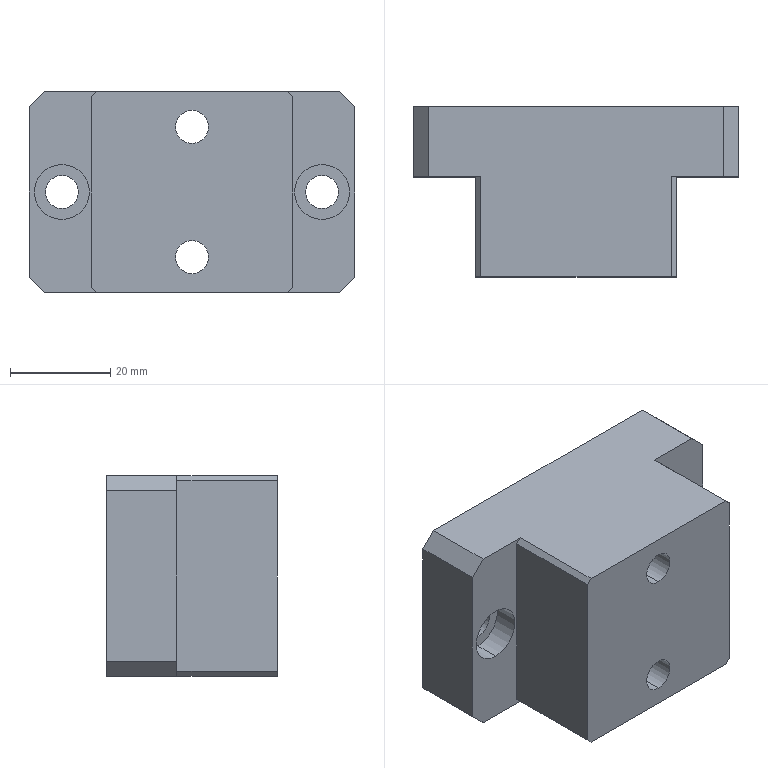Part | SolidWorks | features Chamfer 2, HoleWzd 2, Extrusion 1, ICE 1 | 1 solid | 38 faces | box 65 x 34 x 40 mm | volume 63388 mm3 | plane 22 | cylinder 16 | commonest cylinder face diameters 6.6 x8 11 x8
STEP:
#1=CARTESIAN_POINT('',(26.,8.,5.5));
#2=VERTEX_POINT('',#1);
#3=CARTESIAN_POINT('',(26.,8.,-5.5));
#4=VERTEX_POINT('',#3);
#5=CARTESIAN_POINT('',(26.,8.,0.));
#6=DIRECTION('',(0.,-1.,0.));
#7=DIRECTION('',(0.,0.,-1.));
#8=AXIS2_PLACEMENT_3D('',#5,#6,#7);
#9=CIRCLE('',#8,5.5);
#10=EDGE_CURVE('',#2,#4,#9,.T.);
#11=ORIENTED_EDGE('',*,*,#10,.F.);
#12=CARTESIAN_POINT('',(26.,3.,5.5));
#13=VERTEX_POINT('',#12);
#14=CARTESIAN_POINT('',(26.,3.,5.5));
#15=DIRECTION('',(0.,-1.,0.));
#16=VECTOR('',#15,1000.);
#17=LINE('',#14,#16);
#18=EDGE_CURVE('',#2,#13,#17,.T.);
#19=ORIENTED_EDGE('',*,*,#18,.T.);
#20=CARTESIAN_POINT('',(26.,3.,-5.5));
#21=VERTEX_POINT('',#20);
#22=CARTESIAN_POINT('',(26.,3.,0.));
#23=DIRECTION('',(0.,-1.,0.));
#24=DIRECTION('',(0.,0.,-1.));
#25=AXIS2_PLACEMENT_3D('',#22,#23,#24);
#26=CIRCLE('',#25,5.5);
#27=EDGE_CURVE('',#13,#21,#26,.T.);
#28=ORIENTED_EDGE('',*,*,#27,.T.);
#29=CARTESIAN_POINT('',(26.,3.,-5.5));
#30=DIRECTION('',(0.,-1.,0.));
#31=VECTOR('',#30,1000.);
#32=LINE('',#29,#31);
#33=EDGE_CURVE('',#4,#21,#32,.T.);
#34=ORIENTED_EDGE('',*,*,#33,.F.);
#35=EDGE_LOOP('',(#11,#19,#28,#34));
#36=FACE_OUTER_BOUND('',#35,.T.);
#37=CARTESIAN_POINT('',(26.,3.,0.));
#38=DIRECTION('',(0.,-1.,0.));
#39=DIRECTION('',(0.,0.,-1.));
#40=AXIS2_PLACEMENT_3D('',#37,#38,#39);
#41=CYLINDRICAL_SURFACE('',#40,5.5);
#42=ADVANCED_FACE('',(#36),#41,.F.);
#43=CARTESIAN_POINT('',(26.,17.,3.3));
#44=VERTEX_POINT('',#43);
#45=CARTESIAN_POINT('',(26.,17.,-3.3));
#46=VERTEX_POINT('',#45);
#47=CARTESIAN_POINT('',(26.,17.,0.));
#48=DIRECTION('',(0.,-1.,0.));
#49=DIRECTION('',(0.,0.,-1.));
#50=AXIS2_PLACEMENT_3D('',#47,#48,#49);
#51=CIRCLE('',#50,3.3);
#52=EDGE_CURVE('',#44,#46,#51,.T.);
#53=ORIENTED_EDGE('',*,*,#52,.F.);
#54=CARTESIAN_POINT('',(26.,8.,3.3));
#55=VERTEX_POINT('',#54);
#56=CARTESIAN_POINT('',(26.,3.,3.3));
#57=DIRECTION('',(0.,-1.,0.));
#58=VECTOR('',#57,1000.);
#59=LINE('',#56,#58);
#60=EDGE_CURVE('',#44,#55,#59,.T.);
#61=ORIENTED_EDGE('',*,*,#60,.T.);
#62=CARTESIAN_POINT('',(26.,8.,-3.3));
#63=VERTEX_POINT('',#62);
#64=CARTESIAN_POINT('',(26.,8.,0.));
#65=DIRECTION('',(0.,-1.,0.));
#66=DIRECTION('',(0.,0.,-1.));
#67=AXIS2_PLACEMENT_3D('',#64,#65,#66);
#68=CIRCLE('',#67,3.3);
#69=EDGE_CURVE('',#55,#63,#68,.T.);
#70=ORIENTED_EDGE('',*,*,#69,.T.);
#71=CARTESIAN_POINT('',(26.,3.,-3.3));
#72=DIRECTION('',(0.,-1.,0.));
#73=VECTOR('',#72,1000.);
#74=LINE('',#71,#73);
#75=EDGE_CURVE('',#46,#63,#74,.T.);
#76=ORIENTED_EDGE('',*,*,#75,.F.);
#77=EDGE_LOOP('',(#53,#61,#70,#76));
#78=FACE_OUTER_BOUND('',#77,.T.);
#79=CARTESIAN_POINT('',(26.,3.,0.));
#80=DIRECTION('',(0.,-1.,0.));
#81=DIRECTION('',(0.,0.,-1.));
#82=AXIS2_PLACEMENT_3D('',#79,#80,#81);
#83=CYLINDRICAL_SURFACE('',#82,3.3);
#84=ADVANCED_FACE('',(#78),#83,.F.);
#85=CARTESIAN_POINT('',(-26.,8.,5.5));
#86=VERTEX_POINT('',#85);
#87=CARTESIAN_POINT('',(-26.,8.,-5.5));
#88=VERTEX_POINT('',#87);
#89=CARTESIAN_POINT('',(-26.,8.,0.));
#90=DIRECTION('',(0.,-1.,0.));
#91=DIRECTION('',(0.,0.,-1.));
#92=AXIS2_PLACEMENT_3D('',#89,#90,#91);
#93=CIRCLE('',#92,5.5);
#94=EDGE_CURVE('',#86,#88,#93,.T.);
#95=ORIENTED_EDGE('',*,*,#94,.F.);
#96=CARTESIAN_POINT('',(-26.,3.,5.5));
#97=VERTEX_POINT('',#96);
#98=CARTESIAN_POINT('',(-26.,3.,5.5));
#99=DIRECTION('',(0.,-1.,0.));
#100=VECTOR('',#99,1000.);
#101=LINE('',#98,#100);
#102=EDGE_CURVE('',#86,#97,#101,.T.);
#103=ORIENTED_EDGE('',*,*,#102,.T.);
#104=CARTESIAN_POINT('',(-26.,3.,-5.5));
#105=VERTEX_POINT('',#104);
#106=CARTESIAN_POINT('',(-26.,3.,0.));
#107=DIRECTION('',(0.,-1.,0.));
#108=DIRECTION('',(0.,0.,-1.));
#109=AXIS2_PLACEMENT_3D('',#106,#107,#108);
#110=CIRCLE('',#109,5.5);
#111=EDGE_CURVE('',#97,#105,#110,.T.);
#112=ORIENTED_EDGE('',*,*,#111,.T.);
#113=CARTESIAN_POINT('',(-26.,3.,-5.5));
#114=DIRECTION('',(0.,-1.,0.));
#115=VECTOR('',#114,1000.);
#116=LINE('',#113,#115);
#117=EDGE_CURVE('',#88,#105,#116,.T.);
#118=ORIENTED_EDGE('',*,*,#117,.F.);
#119=EDGE_LOOP('',(#95,#103,#112,#118));
#120=FACE_OUTER_BOUND('',#119,.T.);
#121=CARTESIAN_POINT('',(-26.,3.,0.));
#122=DIRECTION('',(0.,-1.,0.));
#123=DIRECTION('',(0.,0.,-1.));
#124=AXIS2_PLACEMENT_3D('',#121,#122,#123);
#125=CYLINDRICAL_SURFACE('',#124,5.5);
#126=ADVANCED_FACE('',(#120),#125,.F.);
#127=CARTESIAN_POINT('',(-26.,17.,3.3));
#128=VERTEX_POINT('',#127);
#129=CARTESIAN_POINT('',(-26.,17.,-3.3));
#130=VERTEX_POINT('',#129);
#131=CARTESIAN_POINT('',(-26.,17.,0.));
#132=DIRECTION('',(0.,-1.,0.));
#133=DIRECTION('',(0.,0.,-1.));
#134=AXIS2_PLACEMENT_3D('',#131,#132,#133);
#135=CIRCLE('',#134,3.3);
#136=EDGE_CURVE('',#128,#130,#135,.T.);
#137=ORIENTED_EDGE('',*,*,#136,.F.);
#138=CARTESIAN_POINT('',(-26.,8.,3.3));
#139=VERTEX_POINT('',#138);
#140=CARTESIAN_POINT('',(-26.,3.,3.3));
#141=DIRECTION('',(0.,-1.,0.));
#142=VECTOR('',#141,1000.);
#143=LINE('',#140,#142);
#144=EDGE_CURVE('',#128,#139,#143,.T.);
#145=ORIENTED_EDGE('',*,*,#144,.T.);
#146=CARTESIAN_POINT('',(-26.,8.,-3.3));
#147=VERTEX_POINT('',#146);
#148=CARTESIAN_POINT('',(-26.,8.,0.));
#149=DIRECTION('',(0.,-1.,0.));
#150=DIRECTION('',(0.,0.,-1.));
#151=AXIS2_PLACEMENT_3D('',#148,#149,#150);
#152=CIRCLE('',#151,3.3);
#153=EDGE_CURVE('',#139,#147,#152,.T.);
#154=ORIENTED_EDGE('',*,*,#153,.T.);
#155=CARTESIAN_POINT('',(-26.,3.,-3.3));
#156=DIRECTION('',(0.,-1.,0.));
#157=VECTOR('',#156,1000.);
#158=LINE('',#155,#157);
#159=EDGE_CURVE('',#130,#147,#158,.T.);
#160=ORIENTED_EDGE('',*,*,#159,.F.);
#161=EDGE_LOOP('',(#137,#145,#154,#160));
#162=FACE_OUTER_BOUND('',#161,.T.);
#163=CARTESIAN_POINT('',(-26.,3.,0.));
#164=DIRECTION('',(0.,-1.,0.));
#165=DIRECTION('',(0.,0.,-1.));
#166=AXIS2_PLACEMENT_3D('',#163,#164,#165);
#167=CYLINDRICAL_SURFACE('',#166,3.3);
#168=ADVANCED_FACE('',(#162),#167,.F.);
#169=CARTESIAN_POINT('',(0.,10.2,7.5));
#170=VERTEX_POINT('',#169);
#171=CARTESIAN_POINT('',(0.,10.2,18.5));
#172=VERTEX_POINT('',#171);
#173=CARTESIAN_POINT('',(0.,10.2,13.));
#174=DIRECTION('',(0.,1.,0.));
#175=DIRECTION('',(0.,0.,1.));
#176=AXIS2_PLACEMENT_3D('',#173,#174,#175);
#177=CIRCLE('',#176,5.5);
#178=EDGE_CURVE('',#170,#172,#177,.T.);
#179=ORIENTED_EDGE('',*,*,#178,.F.);
#180=CARTESIAN_POINT('',(0.,17.,7.5));
#181=VERTEX_POINT('',#180);
#182=CARTESIAN_POINT('',(0.,17.,7.5));
#183=DIRECTION('',(0.,1.,0.));
#184=VECTOR('',#183,1000.);
#185=LINE('',#182,#184);
#186=EDGE_CURVE('',#170,#181,#185,.T.);
#187=ORIENTED_EDGE('',*,*,#186,.T.);
#188=CARTESIAN_POINT('',(0.,17.,18.5));
#189=VERTEX_POINT('',#188);
#190=CARTESIAN_POINT('',(0.,17.,13.));
#191=DIRECTION('',(0.,1.,0.));
#192=DIRECTION('',(0.,0.,1.));
#193=AXIS2_PLACEMENT_3D('',#190,#191,#192);
#194=CIRCLE('',#193,5.5);
#195=EDGE_CURVE('',#181,#189,#194,.T.);
#196=ORIENTED_EDGE('',*,*,#195,.T.);
#197=CARTESIAN_POINT('',(0.,17.,18.5));
#198=DIRECTION('',(0.,1.,0.));
#199=VECTOR('',#198,1000.);
#200=LINE('',#197,#199);
#201=EDGE_CURVE('',#172,#189,#200,.T.);
#202=ORIENTED_EDGE('',*,*,#201,.F.);
#203=EDGE_LOOP('',(#179,#187,#196,#202));
#204=FACE_OUTER_BOUND('',#203,.T.);
#205=CARTESIAN_POINT('',(0.,17.,13.));
#206=DIRECTION('',(0.,1.,0.));
#207=DIRECTION('',(0.,0.,1.));
#208=AXIS2_PLACEMENT_3D('',#205,#206,#207);
#209=CYLINDRICAL_SURFACE('',#208,5.5);
#210=ADVANCED_FACE('',(#204),#209,.F.);
#211=CARTESIAN_POINT('',(0.,-17.,9.7));
#212=VERTEX_POINT('',#211);
#213=CARTESIAN_POINT('',(0.,-17.,16.3));
#214=VERTEX_POINT('',#213);
#215=CARTESIAN_POINT('',(0.,-17.,13.));
#216=DIRECTION('',(0.,1.,0.));
#217=DIRECTION('',(0.,0.,1.));
#218=AXIS2_PLACEMENT_3D('',#215,#216,#217);
#219=CIRCLE('',#218,3.3);
#220=EDGE_CURVE('',#212,#214,#219,.T.);
#221=ORIENTED_EDGE('',*,*,#220,.F.);
#222=CARTESIAN_POINT('',(0.,10.2,9.7));
#223=VERTEX_POINT('',#222);
#224=CARTESIAN_POINT('',(0.,17.,9.7));
#225=DIRECTION('',(0.,1.,0.));
#226=VECTOR('',#225,1000.);
#227=LINE('',#224,#226);
#228=EDGE_CURVE('',#212,#223,#227,.T.);
#229=ORIENTED_EDGE('',*,*,#228,.T.);
#230=CARTESIAN_POINT('',(0.,10.2,16.3));
#231=VERTEX_POINT('',#230);
#232=CARTESIAN_POINT('',(0.,10.2,13.));
#233=DIRECTION('',(0.,1.,0.));
#234=DIRECTION('',(0.,0.,1.));
#235=AXIS2_PLACEMENT_3D('',#232,#233,#234);
#236=CIRCLE('',#235,3.3);
#237=EDGE_CURVE('',#223,#231,#236,.T.);
#238=ORIENTED_EDGE('',*,*,#237,.T.);
#239=CARTESIAN_POINT('',(0.,17.,16.3));
#240=DIRECTION('',(0.,1.,0.));
#241=VECTOR('',#240,1000.);
#242=LINE('',#239,#241);
#243=EDGE_CURVE('',#214,#231,#242,.T.);
#244=ORIENTED_EDGE('',*,*,#243,.F.);
#245=EDGE_LOOP('',(#221,#229,#238,#244));
#246=FACE_OUTER_BOUND('',#245,.T.);
#247=CARTESIAN_POINT('',(0.,17.,13.));
#248=DIRECTION('',(0.,1.,0.));
#249=DIRECTION('',(0.,0.,1.));
#250=AXIS2_PLACEMENT_3D('',#247,#248,#249);
#251=CYLINDRICAL_SURFACE('',#250,3.3);
#252=ADVANCED_FACE('',(#246),#251,.F.);
#253=CARTESIAN_POINT('',(0.,10.2,-18.5));
#254=VERTEX_POINT('',#253);
#255=CARTESIAN_POINT('',(0.,10.2,-7.5));
#256=VERTEX_POINT('',#255);
#257=CARTESIAN_POINT('',(0.,10.2,-13.));
#258=DIRECTION('',(0.,1.,0.));
#259=DIRECTION('',(0.,0.,1.));
#260=AXIS2_PLACEMENT_3D('',#257,#258,#259);
#261=CIRCLE('',#260,5.5);
#262=EDGE_CURVE('',#254,#256,#261,.T.);
#263=ORIENTED_EDGE('',*,*,#262,.F.);
#264=CARTESIAN_POINT('',(0.,17.,-18.5));
#265=VERTEX_POINT('',#264);
#266=CARTESIAN_POINT('',(0.,17.,-18.5));
#267=DIRECTION('',(0.,1.,0.));
#268=VECTOR('',#267,1000.);
#269=LINE('',#266,#268);
#270=EDGE_CURVE('',#254,#265,#269,.T.);
#271=ORIENTED_EDGE('',*,*,#270,.T.);
#272=CARTESIAN_POINT('',(0.,17.,-7.5));
#273=VERTEX_POINT('',#272);
#274=CARTESIAN_POINT('',(0.,17.,-13.));
#275=DIRECTION('',(0.,1.,0.));
#276=DIRECTION('',(0.,0.,1.));
#277=AXIS2_PLACEMENT_3D('',#274,#275,#276);
#278=CIRCLE('',#277,5.5);
#279=EDGE_CURVE('',#265,#273,#278,.T.);
#280=ORIENTED_EDGE('',*,*,#279,.T.);
#281=CARTESIAN_POINT('',(0.,17.,-7.5));
#282=DIRECTION('',(0.,1.,0.));
#283=VECTOR('',#282,1000.);
#284=LINE('',#281,#283);
#285=EDGE_CURVE('',#256,#273,#284,.T.);
#286=ORIENTED_EDGE('',*,*,#285,.F.);
#287=EDGE_LOOP('',(#263,#271,#280,#286));
#288=FACE_OUTER_BOUND('',#287,.T.);
#289=CARTESIAN_POINT('',(0.,17.,-13.));
#290=DIRECTION('',(0.,1.,0.));
#291=DIRECTION('',(0.,0.,1.));
#292=AXIS2_PLACEMENT_3D('',#289,#290,#291);
#293=CYLINDRICAL_SURFACE('',#292,5.5);
#294=ADVANCED_FACE('',(#288),#293,.F.);
#295=CARTESIAN_POINT('',(0.,-17.,-16.3));
#296=VERTEX_POINT('',#295);
#297=CARTESIAN_POINT('',(0.,-17.,-9.7));
#298=VERTEX_POINT('',#297);
#299=CARTESIAN_POINT('',(0.,-17.,-13.));
#300=DIRECTION('',(0.,1.,0.));
#301=DIRECTION('',(0.,0.,1.));
#302=AXIS2_PLACEMENT_3D('',#299,#300,#301);
#303=CIRCLE('',#302,3.3);
#304=EDGE_CURVE('',#296,#298,#303,.T.);
#305=ORIENTED_EDGE('',*,*,#304,.F.);
#306=CARTESIAN_POINT('',(0.,10.2,-16.3));
#307=VERTEX_POINT('',#306);
#308=CARTESIAN_POINT('',(0.,17.,-16.3));
#309=DIRECTION('',(0.,1.,0.));
#310=VECTOR('',#309,1000.);
#311=LINE('',#308,#310);
#312=EDGE_CURVE('',#296,#307,#311,.T.);
#313=ORIENTED_EDGE('',*,*,#312,.T.);
#314=CARTESIAN_POINT('',(0.,10.2,-9.7));
#315=VERTEX_POINT('',#314);
#316=CARTESIAN_POINT('',(0.,10.2,-13.));
#317=DIRECTION('',(0.,1.,0.));
#318=DIRECTION('',(0.,0.,1.));
#319=AXIS2_PLACEMENT_3D('',#316,#317,#318);
#320=CIRCLE('',#319,3.3);
#321=EDGE_CURVE('',#307,#315,#320,.T.);
#322=ORIENTED_EDGE('',*,*,#321,.T.);
#323=CARTESIAN_POINT('',(0.,17.,-9.7));
#324=DIRECTION('',(0.,1.,0.));
#325=VECTOR('',#324,1000.);
#326=LINE('',#323,#325);
#327=EDGE_CURVE('',#298,#315,#326,.T.);
#328=ORIENTED_EDGE('',*,*,#327,.F.);
#329=EDGE_LOOP('',(#305,#313,#322,#328));
#330=FACE_OUTER_BOUND('',#329,.T.);
#331=CARTESIAN_POINT('',(0.,17.,-13.));
#332=DIRECTION('',(0.,1.,0.));
#333=DIRECTION('',(0.,0.,1.));
#334=AXIS2_PLACEMENT_3D('',#331,#332,#333);
#335=CYLINDRICAL_SURFACE('',#334,3.3);
#336=ADVANCED_FACE('',(#330),#335,.F.);
#337=CARTESIAN_POINT('',(32.5,3.,-17.));
#338=VERTEX_POINT('',#337);
#339=CARTESIAN_POINT('',(32.5,3.,17.));
#340=VERTEX_POINT('',#339);
#341=CARTESIAN_POINT('',(32.5,3.,20.));
#342=DIRECTION('',(0.,0.,1.));
#343=VECTOR('',#342,1000.);
#344=LINE('',#341,#343);
#345=EDGE_CURVE('',#338,#340,#344,.T.);
#346=ORIENTED_EDGE('',*,*,#345,.F.);
#347=CARTESIAN_POINT('',(32.5,17.,-17.));
#348=VERTEX_POINT('',#347);
#349=CARTESIAN_POINT('',(32.5,17.,-17.));
#350=DIRECTION('',(0.,1.,0.));
#351=VECTOR('',#350,1000.);
#352=LINE('',#349,#351);
#353=EDGE_CURVE('',#338,#348,#352,.T.);
#354=ORIENTED_EDGE('',*,*,#353,.T.);
#355=CARTESIAN_POINT('',(32.5,17.,17.));
#356=VERTEX_POINT('',#355);
#357=CARTESIAN_POINT('',(32.5,17.,20.));
#358=DIRECTION('',(0.,0.,-1.));
#359=VECTOR('',#358,1000.);
#360=LINE('',#357,#359);
#361=EDGE_CURVE('',#356,#348,#360,.T.);
#362=ORIENTED_EDGE('',*,*,#361,.F.);
#363=CARTESIAN_POINT('',(32.5,17.,17.));
#364=DIRECTION('',(0.,-1.,0.));
#365=VECTOR('',#364,1000.);
#366=LINE('',#363,#365);
#367=EDGE_CURVE('',#356,#340,#366,.T.);
#368=ORIENTED_EDGE('',*,*,#367,.T.);
#369=EDGE_LOOP('',(#346,#354,#362,#368));
#370=FACE_OUTER_BOUND('',#369,.T.);
#371=CARTESIAN_POINT('',(32.5,17.,20.));
#372=DIRECTION('',(-1.,0.,0.));
#373=DIRECTION('',(0.,0.,1.));
#374=AXIS2_PLACEMENT_3D('',#371,#372,#373);
#375=PLANE('',#374);
#376=ADVANCED_FACE('',(#370),#375,.F.);
#377=CARTESIAN_POINT('',(19.,-17.,-20.));
#378=VERTEX_POINT('',#377);
#379=CARTESIAN_POINT('',(-19.,-17.,-20.));
#380=VERTEX_POINT('',#379);
#381=CARTESIAN_POINT('',(-32.5,-17.,-20.));
#382=DIRECTION('',(-1.,0.,0.));
#383=VECTOR('',#382,1000.);
#384=LINE('',#381,#383);
#385=EDGE_CURVE('',#378,#380,#384,.T.);
#386=ORIENTED_EDGE('',*,*,#385,.T.);
#387=CARTESIAN_POINT('',(-19.,3.,-20.));
#388=VERTEX_POINT('',#387);
#389=CARTESIAN_POINT('',(-19.,3.,-20.));
#390=DIRECTION('',(0.,1.,0.));
#391=VECTOR('',#390,1000.);
#392=LINE('',#389,#391);
#393=EDGE_CURVE('',#380,#388,#392,.T.);
#394=ORIENTED_EDGE('',*,*,#393,.T.);
#395=CARTESIAN_POINT('',(-29.5,3.,-20.));
#396=VERTEX_POINT('',#395);
#397=CARTESIAN_POINT('',(-32.5,3.,-20.));
#398=DIRECTION('',(1.,0.,0.));
#399=VECTOR('',#398,1000.);
#400=LINE('',#397,#399);
#401=EDGE_CURVE('',#396,#388,#400,.T.);
#402=ORIENTED_EDGE('',*,*,#401,.F.);
#403=CARTESIAN_POINT('',(-29.5,17.,-20.));
#404=VERTEX_POINT('',#403);
#405=CARTESIAN_POINT('',(-29.5,17.,-20.));
#406=DIRECTION('',(0.,1.,0.));
#407=VECTOR('',#406,1000.);
#408=LINE('',#405,#407);
#409=EDGE_CURVE('',#396,#404,#408,.T.);
#410=ORIENTED_EDGE('',*,*,#409,.T.);
#411=CARTESIAN_POINT('',(29.5,17.,-20.));
#412=VERTEX_POINT('',#411);
#413=CARTESIAN_POINT('',(-32.5,17.,-20.));
#414=DIRECTION('',(-1.,0.,0.));
#415=VECTOR('',#414,1000.);
#416=LINE('',#413,#415);
#417=EDGE_CURVE('',#412,#404,#416,.T.);
#418=ORIENTED_EDGE('',*,*,#417,.F.);
#419=CARTESIAN_POINT('',(29.5,3.,-20.));
#420=VERTEX_POINT('',#419);
#421=CARTESIAN_POINT('',(29.5,17.,-20.));
#422=DIRECTION('',(0.,-1.,0.));
#423=VECTOR('',#422,1000.);
#424=LINE('',#421,#423);
#425=EDGE_CURVE('',#412,#420,#424,.T.);
#426=ORIENTED_EDGE('',*,*,#425,.T.);
#427=CARTESIAN_POINT('',(19.,3.,-20.));
#428=VERTEX_POINT('',#427);
#429=CARTESIAN_POINT('',(-32.5,3.,-20.));
#430=DIRECTION('',(1.,0.,0.));
#431=VECTOR('',#430,1000.);
#432=LINE('',#429,#431);
#433=EDGE_CURVE('',#428,#420,#432,.T.);
#434=ORIENTED_EDGE('',*,*,#433,.F.);
#435=CARTESIAN_POINT('',(19.,-17.,-20.));
#436=DIRECTION('',(0.,-1.,0.));
#437=VECTOR('',#436,1000.);
#438=LINE('',#435,#437);
#439=EDGE_CURVE('',#428,#378,#438,.T.);
#440=ORIENTED_EDGE('',*,*,#439,.T.);
#441=EDGE_LOOP('',(#386,#394,#402,#410,#418,#426,#434,#440));
#442=FACE_OUTER_BOUND('',#441,.T.);
#443=CARTESIAN_POINT('',(-32.5,17.,-20.));
#444=DIRECTION('',(0.,0.,1.));
#445=DIRECTION('',(1.,0.,0.));
#446=AXIS2_PLACEMENT_3D('',#443,#444,#445);
#447=PLANE('',#446);
#448=ADVANCED_FACE('',(#442),#447,.F.);
#449=CARTESIAN_POINT('',(-32.5,3.,17.));
#450=VERTEX_POINT('',#449);
#451=CARTESIAN_POINT('',(-32.5,3.,-17.));
#452=VERTEX_POINT('',#451);
#453=CARTESIAN_POINT('',(-32.5,3.,20.));
#454=DIRECTION('',(0.,0.,-1.));
#455=VECTOR('',#454,1000.);
#456=LINE('',#453,#455);
#457=EDGE_CURVE('',#450,#452,#456,.T.);
#458=ORIENTED_EDGE('',*,*,#457,.F.);
#459=CARTESIAN_POINT('',(-32.5,17.,17.));
#460=VERTEX_POINT('',#459);
#461=CARTESIAN_POINT('',(-32.5,17.,17.));
#462=DIRECTION('',(0.,1.,0.));
#463=VECTOR('',#462,1000.);
#464=LINE('',#461,#463);
#465=EDGE_CURVE('',#450,#460,#464,.T.);
#466=ORIENTED_EDGE('',*,*,#465,.T.);
#467=CARTESIAN_POINT('',(-32.5,17.,-17.));
#468=VERTEX_POINT('',#467);
#469=CARTESIAN_POINT('',(-32.5,17.,20.));
#470=DIRECTION('',(0.,0.,1.));
#471=VECTOR('',#470,1000.);
#472=LINE('',#469,#471);
#473=EDGE_CURVE('',#468,#460,#472,.T.);
#474=ORIENTED_EDGE('',*,*,#473,.F.);
#475=CARTESIAN_POINT('',(-32.5,17.,-17.));
#476=DIRECTION('',(0.,-1.,0.));
#477=VECTOR('',#476,1000.);
#478=LINE('',#475,#477);
#479=EDGE_CURVE('',#468,#452,#478,.T.);
#480=ORIENTED_EDGE('',*,*,#479,.T.);
#481=EDGE_LOOP('',(#458,#466,#474,#480));
#482=FACE_OUTER_BOUND('',#481,.T.);
#483=CARTESIAN_POINT('',(-32.5,17.,20.));
#484=DIRECTION('',(1.,0.,0.));
#485=DIRECTION('',(0.,0.,-1.));
#486=AXIS2_PLACEMENT_3D('',#483,#484,#485);
#487=PLANE('',#486);
#488=ADVANCED_FACE('',(#482),#487,.F.);
#489=CARTESIAN_POINT('',(-19.,3.,20.));
#490=VERTEX_POINT('',#489);
#491=CARTESIAN_POINT('',(-29.5,3.,20.));
#492=VERTEX_POINT('',#491);
#493=CARTESIAN_POINT('',(-32.5,3.,20.));
#494=DIRECTION('',(-1.,0.,0.));
#495=VECTOR('',#494,1000.);
#496=LINE('',#493,#495);
#497=EDGE_CURVE('',#490,#492,#496,.T.);
#498=ORIENTED_EDGE('',*,*,#497,.F.);
#499=CARTESIAN_POINT('',(-19.,-17.,20.));
#500=VERTEX_POINT('',#499);
#501=CARTESIAN_POINT('',(-19.,-17.,20.));
#502=DIRECTION('',(0.,-1.,0.));
#503=VECTOR('',#502,1000.);
#504=LINE('',#501,#503);
#505=EDGE_CURVE('',#490,#500,#504,.T.);
#506=ORIENTED_EDGE('',*,*,#505,.T.);
#507=CARTESIAN_POINT('',(19.,-17.,20.));
#508=VERTEX_POINT('',#507);
#509=CARTESIAN_POINT('',(-32.5,-17.,20.));
#510=DIRECTION('',(1.,0.,0.));
#511=VECTOR('',#510,1000.);
#512=LINE('',#509,#511);
#513=EDGE_CURVE('',#500,#508,#512,.T.);
#514=ORIENTED_EDGE('',*,*,#513,.T.);
#515=CARTESIAN_POINT('',(19.,3.,20.));
#516=VERTEX_POINT('',#515);
#517=CARTESIAN_POINT('',(19.,3.,20.));
#518=DIRECTION('',(0.,1.,0.));
#519=VECTOR('',#518,1000.);
#520=LINE('',#517,#519);
#521=EDGE_CURVE('',#508,#516,#520,.T.);
#522=ORIENTED_EDGE('',*,*,#521,.T.);
#523=CARTESIAN_POINT('',(29.5,3.,20.));
#524=VERTEX_POINT('',#523);
#525=CARTESIAN_POINT('',(-32.5,3.,20.));
#526=DIRECTION('',(-1.,0.,0.));
#527=VECTOR('',#526,1000.);
#528=LINE('',#525,#527);
#529=EDGE_CURVE('',#524,#516,#528,.T.);
#530=ORIENTED_EDGE('',*,*,#529,.F.);
#531=CARTESIAN_POINT('',(29.5,17.,20.));
#532=VERTEX_POINT('',#531);
#533=CARTESIAN_POINT('',(29.5,17.,20.));
#534=DIRECTION('',(0.,1.,0.));
#535=VECTOR('',#534,1000.);
#536=LINE('',#533,#535);
#537=EDGE_CURVE('',#524,#532,#536,.T.);
#538=ORIENTED_EDGE('',*,*,#537,.T.);
#539=CARTESIAN_POINT('',(-29.5,17.,20.));
#540=VERTEX_POINT('',#539);
#541=CARTESIAN_POINT('',(-32.5,17.,20.));
#542=DIRECTION('',(1.,0.,0.));
#543=VECTOR('',#542,1000.);
#544=LINE('',#541,#543);
#545=EDGE_CURVE('',#540,#532,#544,.T.);
#546=ORIENTED_EDGE('',*,*,#545,.F.);
#547=CARTESIAN_POINT('',(-29.5,17.,20.));
#548=DIRECTION('',(0.,-1.,0.));
#549=VECTOR('',#548,1000.);
#550=LINE('',#547,#549);
#551=EDGE_CURVE('',#540,#492,#550,.T.);
#552=ORIENTED_EDGE('',*,*,#551,.T.);
#553=EDGE_LOOP('',(#498,#506,#514,#522,#530,#538,#546,#552));
#554=FACE_OUTER_BOUND('',#553,.T.);
#555=CARTESIAN_POINT('',(-32.5,17.,20.));
#556=DIRECTION('',(0.,0.,-1.));
#557=DIRECTION('',(-1.,0.,0.));
#558=AXIS2_PLACEMENT_3D('',#555,#556,#557);
#559=PLANE('',#558);
#560=ADVANCED_FACE('',(#554),#559,.F.);
#561=CARTESIAN_POINT('',(0.,-17.,13.));
#562=DIRECTION('',(0.,1.,0.));
#563=DIRECTION('',(0.,0.,1.));
#564=AXIS2_PLACEMENT_3D('',#561,#562,#563);
#565=CIRCLE('',#564,3.3);
#566=EDGE_CURVE('',#214,#212,#565,.T.);
#567=ORIENTED_EDGE('',*,*,#566,.T.);
#568=ORIENTED_EDGE('',*,*,#220,.T.);
#569=EDGE_LOOP('',(#567,#568));
#570=FACE_BOUND('',#569,.T.);
#571=CARTESIAN_POINT('',(0.,-17.,-13.));
#572=DIRECTION('',(0.,1.,0.));
#573=DIRECTION('',(0.,0.,1.));
#574=AXIS2_PLACEMENT_3D('',#571,#572,#573);
#575=CIRCLE('',#574,3.3);
#576=EDGE_CURVE('',#298,#296,#575,.T.);
#577=ORIENTED_EDGE('',*,*,#576,.T.);
#578=ORIENTED_EDGE('',*,*,#304,.T.);
#579=EDGE_LOOP('',(#577,#578));
#580=FACE_BOUND('',#579,.T.);
#581=ORIENTED_EDGE('',*,*,#513,.F.);
#582=CARTESIAN_POINT('',(-20.,-17.,19.));
#583=VERTEX_POINT('',#582);
#584=CARTESIAN_POINT('',(-19.5,-17.,19.5));
#585=DIRECTION('',(-0.7071,0.,-0.7071));
#586=VECTOR('',#585,1000.);
#587=LINE('',#584,#586);
#588=EDGE_CURVE('',#500,#583,#587,.T.);
#589=ORIENTED_EDGE('',*,*,#588,.T.);
#590=CARTESIAN_POINT('',(-20.,-17.,-19.));
#591=VERTEX_POINT('',#590);
#592=CARTESIAN_POINT('',(-20.,-17.,-20.));
#593=DIRECTION('',(0.,0.,-1.));
#594=VECTOR('',#593,1000.);
#595=LINE('',#592,#594);
#596=EDGE_CURVE('',#583,#591,#595,.T.);
#597=ORIENTED_EDGE('',*,*,#596,.T.);
#598=CARTESIAN_POINT('',(-19.5,-17.,-19.5));
#599=DIRECTION('',(0.7071,0.,-0.7071));
#600=VECTOR('',#599,1000.);
#601=LINE('',#598,#600);
#602=EDGE_CURVE('',#591,#380,#601,.T.);
#603=ORIENTED_EDGE('',*,*,#602,.T.);
#604=ORIENTED_EDGE('',*,*,#385,.F.);
#605=CARTESIAN_POINT('',(20.,-17.,-19.));
#606=VERTEX_POINT('',#605);
#607=CARTESIAN_POINT('',(19.5,-17.,-19.5));
#608=DIRECTION('',(0.7071,0.,0.7071));
#609=VECTOR('',#608,1000.);
#610=LINE('',#607,#609);
#611=EDGE_CURVE('',#378,#606,#610,.T.);
#612=ORIENTED_EDGE('',*,*,#611,.T.);
#613=CARTESIAN_POINT('',(20.,-17.,19.));
#614=VERTEX_POINT('',#613);
#615=CARTESIAN_POINT('',(20.,-17.,-20.));
#616=DIRECTION('',(0.,0.,1.));
#617=VECTOR('',#616,1000.);
#618=LINE('',#615,#617);
#619=EDGE_CURVE('',#606,#614,#618,.T.);
#620=ORIENTED_EDGE('',*,*,#619,.T.);
#621=CARTESIAN_POINT('',(19.5,-17.,19.5));
#622=DIRECTION('',(-0.7071,0.,0.7071));
#623=VECTOR('',#622,1000.);
#624=LINE('',#621,#623);
#625=EDGE_CURVE('',#614,#508,#624,.T.);
#626=ORIENTED_EDGE('',*,*,#625,.T.);
#627=EDGE_LOOP('',(#581,#589,#597,#603,#604,#612,#620,#626));
#628=FACE_OUTER_BOUND('',#627,.T.);
#629=CARTESIAN_POINT('',(0.,-17.,0.));
#630=DIRECTION('',(0.,-1.,0.));
#631=DIRECTION('',(0.,0.,-1.));
#632=AXIS2_PLACEMENT_3D('',#629,#630,#631);
#633=PLANE('',#632);
#634=ADVANCED_FACE('',(#570,#580,#628),#633,.T.);
#635=ORIENTED_EDGE('',*,*,#537,.F.);
#636=CARTESIAN_POINT('',(32.5,3.,17.));
#637=DIRECTION('',(0.7071,0.,-0.7071));
#638=VECTOR('',#637,1000.);
#639=LINE('',#636,#638);
#640=EDGE_CURVE('',#524,#340,#639,.T.);
#641=ORIENTED_EDGE('',*,*,#640,.T.);
#642=ORIENTED_EDGE('',*,*,#367,.F.);
#643=CARTESIAN_POINT('',(32.5,17.,17.));
#644=DIRECTION('',(0.7071,0.,-0.7071));
#645=VECTOR('',#644,1000.);
#646=LINE('',#643,#645);
#647=EDGE_CURVE('',#532,#356,#646,.T.);
#648=ORIENTED_EDGE('',*,*,#647,.F.);
#649=EDGE_LOOP('',(#635,#641,#642,#648));
#650=FACE_OUTER_BOUND('',#649,.T.);
#651=CARTESIAN_POINT('',(32.5,17.,17.));
#652=DIRECTION('',(-0.7071,0.,-0.7071));
#653=DIRECTION('',(0.,-1.,0.));
#654=AXIS2_PLACEMENT_3D('',#651,#652,#653);
#655=PLANE('',#654);
#656=ADVANCED_FACE('',(#650),#655,.F.);
#657=ORIENTED_EDGE('',*,*,#353,.F.);
#658=CARTESIAN_POINT('',(29.5,3.,-20.));
#659=DIRECTION('',(-0.7071,0.,-0.7071));
#660=VECTOR('',#659,1000.);
#661=LINE('',#658,#660);
#662=EDGE_CURVE('',#338,#420,#661,.T.);
#663=ORIENTED_EDGE('',*,*,#662,.T.);
#664=ORIENTED_EDGE('',*,*,#425,.F.);
#665=CARTESIAN_POINT('',(29.5,17.,-20.));
#666=DIRECTION('',(-0.7071,0.,-0.7071));
#667=VECTOR('',#666,1000.);
#668=LINE('',#665,#667);
#669=EDGE_CURVE('',#348,#412,#668,.T.);
#670=ORIENTED_EDGE('',*,*,#669,.F.);
#671=EDGE_LOOP('',(#657,#663,#664,#670));
#672=FACE_OUTER_BOUND('',#671,.T.);
#673=CARTESIAN_POINT('',(29.5,17.,-20.));
#674=DIRECTION('',(-0.7071,0.,0.7071));
#675=DIRECTION('',(0.,-1.,0.));
#676=AXIS2_PLACEMENT_3D('',#673,#674,#675);
#677=PLANE('',#676);
#678=ADVANCED_FACE('',(#672),#677,.F.);
#679=ORIENTED_EDGE('',*,*,#409,.F.);
#680=CARTESIAN_POINT('',(-32.5,3.,-17.));
#681=DIRECTION('',(-0.7071,0.,0.7071));
#682=VECTOR('',#681,1000.);
#683=LINE('',#680,#682);
#684=EDGE_CURVE('',#396,#452,#683,.T.);
#685=ORIENTED_EDGE('',*,*,#684,.T.);
#686=ORIENTED_EDGE('',*,*,#479,.F.);
#687=CARTESIAN_POINT('',(-32.5,17.,-17.));
#688=DIRECTION('',(-0.7071,0.,0.7071));
#689=VECTOR('',#688,1000.);
#690=LINE('',#687,#689);
#691=EDGE_CURVE('',#404,#468,#690,.T.);
#692=ORIENTED_EDGE('',*,*,#691,.F.);
#693=EDGE_LOOP('',(#679,#685,#686,#692));
#694=FACE_OUTER_BOUND('',#693,.T.);
#695=CARTESIAN_POINT('',(-32.5,17.,-17.));
#696=DIRECTION('',(0.7071,0.,0.7071));
#697=DIRECTION('',(0.,-1.,0.));
#698=AXIS2_PLACEMENT_3D('',#695,#696,#697);
#699=PLANE('',#698);
#700=ADVANCED_FACE('',(#694),#699,.F.);
#701=ORIENTED_EDGE('',*,*,#465,.F.);
#702=CARTESIAN_POINT('',(-29.5,3.,20.));
#703=DIRECTION('',(0.7071,0.,0.7071));
#704=VECTOR('',#703,1000.);
#705=LINE('',#702,#704);
#706=EDGE_CURVE('',#450,#492,#705,.T.);
#707=ORIENTED_EDGE('',*,*,#706,.T.);
#708=ORIENTED_EDGE('',*,*,#551,.F.);
#709=CARTESIAN_POINT('',(-29.5,17.,20.));
#710=DIRECTION('',(0.7071,0.,0.7071));
#711=VECTOR('',#710,1000.);
#712=LINE('',#709,#711);
#713=EDGE_CURVE('',#460,#540,#712,.T.);
#714=ORIENTED_EDGE('',*,*,#713,.F.);
#715=EDGE_LOOP('',(#701,#707,#708,#714));
#716=FACE_OUTER_BOUND('',#715,.T.);
#717=CARTESIAN_POINT('',(-29.5,17.,20.));
#718=DIRECTION('',(0.7071,0.,-0.7071));
#719=DIRECTION('',(0.,-1.,0.));
#720=AXIS2_PLACEMENT_3D('',#717,#718,#719);
#721=PLANE('',#720);
#722=ADVANCED_FACE('',(#716),#721,.F.);
#723=CARTESIAN_POINT('',(26.,17.,0.));
#724=DIRECTION('',(0.,-1.,0.));
#725=DIRECTION('',(0.,0.,-1.));
#726=AXIS2_PLACEMENT_3D('',#723,#724,#725);
#727=CIRCLE('',#726,3.3);
#728=EDGE_CURVE('',#46,#44,#727,.T.);
#729=ORIENTED_EDGE('',*,*,#728,.T.);
#730=ORIENTED_EDGE('',*,*,#52,.T.);
#731=EDGE_LOOP('',(#729,#730));
#732=FACE_BOUND('',#731,.T.);
#733=CARTESIAN_POINT('',(-26.,17.,0.));
#734=DIRECTION('',(0.,-1.,0.));
#735=DIRECTION('',(0.,0.,-1.));
#736=AXIS2_PLACEMENT_3D('',#733,#734,#735);
#737=CIRCLE('',#736,3.3);
#738=EDGE_CURVE('',#130,#128,#737,.T.);
#739=ORIENTED_EDGE('',*,*,#738,.T.);
#740=ORIENTED_EDGE('',*,*,#136,.T.);
#741=EDGE_LOOP('',(#739,#740));
#742=FACE_BOUND('',#741,.T.);
#743=CARTESIAN_POINT('',(0.,17.,13.));
#744=DIRECTION('',(0.,1.,0.));
#745=DIRECTION('',(0.,0.,1.));
#746=AXIS2_PLACEMENT_3D('',#743,#744,#745);
#747=CIRCLE('',#746,5.5);
#748=EDGE_CURVE('',#189,#181,#747,.T.);
#749=ORIENTED_EDGE('',*,*,#748,.F.);
#750=ORIENTED_EDGE('',*,*,#195,.F.);
#751=EDGE_LOOP('',(#749,#750));
#752=FACE_BOUND('',#751,.T.);
#753=CARTESIAN_POINT('',(0.,17.,-13.));
#754=DIRECTION('',(0.,1.,0.));
#755=DIRECTION('',(0.,0.,1.));
#756=AXIS2_PLACEMENT_3D('',#753,#754,#755);
#757=CIRCLE('',#756,5.5);
#758=EDGE_CURVE('',#273,#265,#757,.T.);
#759=ORIENTED_EDGE('',*,*,#758,.F.);
#760=ORIENTED_EDGE('',*,*,#279,.F.);
#761=EDGE_LOOP('',(#759,#760));
#762=FACE_BOUND('',#761,.T.);
#763=ORIENTED_EDGE('',*,*,#545,.T.);
#764=ORIENTED_EDGE('',*,*,#647,.T.);
#765=ORIENTED_EDGE('',*,*,#361,.T.);
#766=ORIENTED_EDGE('',*,*,#669,.T.);
#767=ORIENTED_EDGE('',*,*,#417,.T.);
#768=ORIENTED_EDGE('',*,*,#691,.T.);
#769=ORIENTED_EDGE('',*,*,#473,.T.);
#770=ORIENTED_EDGE('',*,*,#713,.T.);
#771=EDGE_LOOP('',(#763,#764,#765,#766,#767,#768,#769,#770));
#772=FACE_OUTER_BOUND('',#771,.T.);
#773=CARTESIAN_POINT('',(0.,17.,0.));
#774=DIRECTION('',(0.,-1.,0.));
#775=DIRECTION('',(0.,0.,-1.));
#776=AXIS2_PLACEMENT_3D('',#773,#774,#775);
#777=PLANE('',#776);
#778=ADVANCED_FACE('',(#732,#742,#752,#762,#772),#777,.F.);
#779=ORIENTED_EDGE('',*,*,#312,.F.);
#780=ORIENTED_EDGE('',*,*,#576,.F.);
#781=ORIENTED_EDGE('',*,*,#327,.T.);
#782=CARTESIAN_POINT('',(0.,10.2,-13.));
#783=DIRECTION('',(0.,1.,0.));
#784=DIRECTION('',(0.,0.,1.));
#785=AXIS2_PLACEMENT_3D('',#782,#783,#784);
#786=CIRCLE('',#785,3.3);
#787=EDGE_CURVE('',#315,#307,#786,.T.);
#788=ORIENTED_EDGE('',*,*,#787,.T.);
#789=EDGE_LOOP('',(#779,#780,#781,#788));
#790=FACE_OUTER_BOUND('',#789,.T.);
#791=CARTESIAN_POINT('',(0.,17.,-13.));
#792=DIRECTION('',(0.,1.,0.));
#793=DIRECTION('',(0.,0.,1.));
#794=AXIS2_PLACEMENT_3D('',#791,#792,#793);
#795=CYLINDRICAL_SURFACE('',#794,3.3);
#796=ADVANCED_FACE('',(#790),#795,.F.);
#797=ORIENTED_EDGE('',*,*,#787,.F.);
#798=ORIENTED_EDGE('',*,*,#321,.F.);
#799=EDGE_LOOP('',(#797,#798));
#800=FACE_BOUND('',#799,.T.);
#801=CARTESIAN_POINT('',(0.,10.2,-13.));
#802=DIRECTION('',(0.,1.,0.));
#803=DIRECTION('',(0.,0.,1.));
#804=AXIS2_PLACEMENT_3D('',#801,#802,#803);
#805=CIRCLE('',#804,5.5);
#806=EDGE_CURVE('',#256,#254,#805,.T.);
#807=ORIENTED_EDGE('',*,*,#806,.T.);
#808=ORIENTED_EDGE('',*,*,#262,.T.);
#809=EDGE_LOOP('',(#807,#808));
#810=FACE_OUTER_BOUND('',#809,.T.);
#811=CARTESIAN_POINT('',(3.3,10.2,-13.));
#812=DIRECTION('',(0.,-1.,0.));
#813=DIRECTION('',(0.,0.,-1.));
#814=AXIS2_PLACEMENT_3D('',#811,#812,#813);
#815=PLANE('',#814);
#816=ADVANCED_FACE('',(#800,#810),#815,.F.);
#817=ORIENTED_EDGE('',*,*,#270,.F.);
#818=ORIENTED_EDGE('',*,*,#806,.F.);
#819=ORIENTED_EDGE('',*,*,#285,.T.);
#820=ORIENTED_EDGE('',*,*,#758,.T.);
#821=EDGE_LOOP('',(#817,#818,#819,#820));
#822=FACE_OUTER_BOUND('',#821,.T.);
#823=CARTESIAN_POINT('',(0.,17.,-13.));
#824=DIRECTION('',(0.,1.,0.));
#825=DIRECTION('',(0.,0.,1.));
#826=AXIS2_PLACEMENT_3D('',#823,#824,#825);
#827=CYLINDRICAL_SURFACE('',#826,5.5);
#828=ADVANCED_FACE('',(#822),#827,.F.);
#829=ORIENTED_EDGE('',*,*,#228,.F.);
#830=ORIENTED_EDGE('',*,*,#566,.F.);
#831=ORIENTED_EDGE('',*,*,#243,.T.);
#832=CARTESIAN_POINT('',(0.,10.2,13.));
#833=DIRECTION('',(0.,1.,0.));
#834=DIRECTION('',(0.,0.,1.));
#835=AXIS2_PLACEMENT_3D('',#832,#833,#834);
#836=CIRCLE('',#835,3.3);
#837=EDGE_CURVE('',#231,#223,#836,.T.);
#838=ORIENTED_EDGE('',*,*,#837,.T.);
#839=EDGE_LOOP('',(#829,#830,#831,#838));
#840=FACE_OUTER_BOUND('',#839,.T.);
#841=CARTESIAN_POINT('',(0.,17.,13.));
#842=DIRECTION('',(0.,1.,0.));
#843=DIRECTION('',(0.,0.,1.));
#844=AXIS2_PLACEMENT_3D('',#841,#842,#843);
#845=CYLINDRICAL_SURFACE('',#844,3.3);
#846=ADVANCED_FACE('',(#840),#845,.F.);
#847=ORIENTED_EDGE('',*,*,#837,.F.);
#848=ORIENTED_EDGE('',*,*,#237,.F.);
#849=EDGE_LOOP('',(#847,#848));
#850=FACE_BOUND('',#849,.T.);
#851=CARTESIAN_POINT('',(0.,10.2,13.));
#852=DIRECTION('',(0.,1.,0.));
#853=DIRECTION('',(0.,0.,1.));
#854=AXIS2_PLACEMENT_3D('',#851,#852,#853);
#855=CIRCLE('',#854,5.5);
#856=EDGE_CURVE('',#172,#170,#855,.T.);
#857=ORIENTED_EDGE('',*,*,#856,.T.);
#858=ORIENTED_EDGE('',*,*,#178,.T.);
#859=EDGE_LOOP('',(#857,#858));
#860=FACE_OUTER_BOUND('',#859,.T.);
#861=CARTESIAN_POINT('',(3.3,10.2,13.));
#862=DIRECTION('',(0.,-1.,0.));
#863=DIRECTION('',(0.,0.,-1.));
#864=AXIS2_PLACEMENT_3D('',#861,#862,#863);
#865=PLANE('',#864);
#866=ADVANCED_FACE('',(#850,#860),#865,.F.);
#867=ORIENTED_EDGE('',*,*,#186,.F.);
#868=ORIENTED_EDGE('',*,*,#856,.F.);
#869=ORIENTED_EDGE('',*,*,#201,.T.);
#870=ORIENTED_EDGE('',*,*,#748,.T.);
#871=EDGE_LOOP('',(#867,#868,#869,#870));
#872=FACE_OUTER_BOUND('',#871,.T.);
#873=CARTESIAN_POINT('',(0.,17.,13.));
#874=DIRECTION('',(0.,1.,0.));
#875=DIRECTION('',(0.,0.,1.));
#876=AXIS2_PLACEMENT_3D('',#873,#874,#875);
#877=CYLINDRICAL_SURFACE('',#876,5.5);
#878=ADVANCED_FACE('',(#872),#877,.F.);
#879=CARTESIAN_POINT('',(-26.,3.,0.));
#880=DIRECTION('',(0.,-1.,0.));
#881=DIRECTION('',(0.,0.,-1.));
#882=AXIS2_PLACEMENT_3D('',#879,#880,#881);
#883=CIRCLE('',#882,5.5);
#884=EDGE_CURVE('',#105,#97,#883,.T.);
#885=ORIENTED_EDGE('',*,*,#884,.F.);
#886=ORIENTED_EDGE('',*,*,#111,.F.);
#887=EDGE_LOOP('',(#885,#886));
#888=FACE_BOUND('',#887,.T.);
#889=ORIENTED_EDGE('',*,*,#401,.T.);
#890=CARTESIAN_POINT('',(-20.,3.,-19.));
#891=VERTEX_POINT('',#890);
#892=CARTESIAN_POINT('',(-20.,3.,-19.));
#893=DIRECTION('',(-0.7071,0.,0.7071));
#894=VECTOR('',#893,1000.);
#895=LINE('',#892,#894);
#896=EDGE_CURVE('',#388,#891,#895,.T.);
#897=ORIENTED_EDGE('',*,*,#896,.T.);
#898=CARTESIAN_POINT('',(-20.,3.,19.));
#899=VERTEX_POINT('',#898);
#900=CARTESIAN_POINT('',(-20.,3.,-20.));
#901=DIRECTION('',(0.,0.,-1.));
#902=VECTOR('',#901,1000.);
#903=LINE('',#900,#902);
#904=EDGE_CURVE('',#899,#891,#903,.T.);
#905=ORIENTED_EDGE('',*,*,#904,.F.);
#906=CARTESIAN_POINT('',(-19.,3.,20.));
#907=DIRECTION('',(0.7071,0.,0.7071));
#908=VECTOR('',#907,1000.);
#909=LINE('',#906,#908);
#910=EDGE_CURVE('',#899,#490,#909,.T.);
#911=ORIENTED_EDGE('',*,*,#910,.T.);
#912=ORIENTED_EDGE('',*,*,#497,.T.);
#913=ORIENTED_EDGE('',*,*,#706,.F.);
#914=ORIENTED_EDGE('',*,*,#457,.T.);
#915=ORIENTED_EDGE('',*,*,#684,.F.);
#916=EDGE_LOOP('',(#889,#897,#905,#911,#912,#913,#914,#915));
#917=FACE_OUTER_BOUND('',#916,.T.);
#918=CARTESIAN_POINT('',(0.,3.,0.));
#919=DIRECTION('',(0.,-1.,0.));
#920=DIRECTION('',(0.,0.,-1.));
#921=AXIS2_PLACEMENT_3D('',#918,#919,#920);
#922=PLANE('',#921);
#923=ADVANCED_FACE('',(#888,#917),#922,.T.);
#924=ORIENTED_EDGE('',*,*,#596,.F.);
#925=CARTESIAN_POINT('',(-20.,3.,19.));
#926=DIRECTION('',(0.,1.,0.));
#927=VECTOR('',#926,1000.);
#928=LINE('',#925,#927);
#929=EDGE_CURVE('',#583,#899,#928,.T.);
#930=ORIENTED_EDGE('',*,*,#929,.T.);
#931=ORIENTED_EDGE('',*,*,#904,.T.);
#932=CARTESIAN_POINT('',(-20.,-17.,-19.));
#933=DIRECTION('',(0.,-1.,0.));
#934=VECTOR('',#933,1000.);
#935=LINE('',#932,#934);
#936=EDGE_CURVE('',#891,#591,#935,.T.);
#937=ORIENTED_EDGE('',*,*,#936,.T.);
#938=EDGE_LOOP('',(#924,#930,#931,#937));
#939=FACE_OUTER_BOUND('',#938,.T.);
#940=CARTESIAN_POINT('',(-20.,3.,-20.));
#941=DIRECTION('',(-1.,0.,0.));
#942=DIRECTION('',(0.,0.,1.));
#943=AXIS2_PLACEMENT_3D('',#940,#941,#942);
#944=PLANE('',#943);
#945=ADVANCED_FACE('',(#939),#944,.T.);
#946=CARTESIAN_POINT('',(26.,3.,0.));
#947=DIRECTION('',(0.,-1.,0.));
#948=DIRECTION('',(0.,0.,-1.));
#949=AXIS2_PLACEMENT_3D('',#946,#947,#948);
#950=CIRCLE('',#949,5.5);
#951=EDGE_CURVE('',#21,#13,#950,.T.);
#952=ORIENTED_EDGE('',*,*,#951,.F.);
#953=ORIENTED_EDGE('',*,*,#27,.F.);
#954=EDGE_LOOP('',(#952,#953));
#955=FACE_BOUND('',#954,.T.);
#956=ORIENTED_EDGE('',*,*,#529,.T.);
#957=CARTESIAN_POINT('',(20.,3.,19.));
#958=VERTEX_POINT('',#957);
#959=CARTESIAN_POINT('',(20.,3.,19.));
#960=DIRECTION('',(0.7071,0.,-0.7071));
#961=VECTOR('',#960,1000.);
#962=LINE('',#959,#961);
#963=EDGE_CURVE('',#516,#958,#962,.T.);
#964=ORIENTED_EDGE('',*,*,#963,.T.);
#965=CARTESIAN_POINT('',(20.,3.,-19.));
#966=VERTEX_POINT('',#965);
#967=CARTESIAN_POINT('',(20.,3.,-20.));
#968=DIRECTION('',(0.,0.,1.));
#969=VECTOR('',#968,1000.);
#970=LINE('',#967,#969);
#971=EDGE_CURVE('',#966,#958,#970,.T.);
#972=ORIENTED_EDGE('',*,*,#971,.F.);
#973=CARTESIAN_POINT('',(19.,3.,-20.));
#974=DIRECTION('',(-0.7071,0.,-0.7071));
#975=VECTOR('',#974,1000.);
#976=LINE('',#973,#975);
#977=EDGE_CURVE('',#966,#428,#976,.T.);
#978=ORIENTED_EDGE('',*,*,#977,.T.);
#979=ORIENTED_EDGE('',*,*,#433,.T.);
#980=ORIENTED_EDGE('',*,*,#662,.F.);
#981=ORIENTED_EDGE('',*,*,#345,.T.);
#982=ORIENTED_EDGE('',*,*,#640,.F.);
#983=EDGE_LOOP('',(#956,#964,#972,#978,#979,#980,#981,#982));
#984=FACE_OUTER_BOUND('',#983,.T.);
#985=CARTESIAN_POINT('',(0.,3.,0.));
#986=DIRECTION('',(0.,-1.,0.));
#987=DIRECTION('',(0.,0.,-1.));
#988=AXIS2_PLACEMENT_3D('',#985,#986,#987);
#989=PLANE('',#988);
#990=ADVANCED_FACE('',(#955,#984),#989,.T.);
#991=ORIENTED_EDGE('',*,*,#971,.T.);
#992=CARTESIAN_POINT('',(20.,-17.,19.));
#993=DIRECTION('',(0.,-1.,0.));
#994=VECTOR('',#993,1000.);
#995=LINE('',#992,#994);
#996=EDGE_CURVE('',#958,#614,#995,.T.);
#997=ORIENTED_EDGE('',*,*,#996,.T.);
#998=ORIENTED_EDGE('',*,*,#619,.F.);
#999=CARTESIAN_POINT('',(20.,3.,-19.));
#1000=DIRECTION('',(0.,1.,0.));
#1001=VECTOR('',#1000,1000.);
#1002=LINE('',#999,#1001);
#1003=EDGE_CURVE('',#606,#966,#1002,.T.);
#1004=ORIENTED_EDGE('',*,*,#1003,.T.);
#1005=EDGE_LOOP('',(#991,#997,#998,#1004));
#1006=FACE_OUTER_BOUND('',#1005,.T.);
#1007=CARTESIAN_POINT('',(20.,3.,-20.));
#1008=DIRECTION('',(1.,0.,0.));
#1009=DIRECTION('',(0.,0.,-1.));
#1010=AXIS2_PLACEMENT_3D('',#1007,#1008,#1009);
#1011=PLANE('',#1010);
#1012=ADVANCED_FACE('',(#1006),#1011,.T.);
#1013=ORIENTED_EDGE('',*,*,#144,.F.);
#1014=ORIENTED_EDGE('',*,*,#738,.F.);
#1015=ORIENTED_EDGE('',*,*,#159,.T.);
#1016=CARTESIAN_POINT('',(-26.,8.,0.));
#1017=DIRECTION('',(0.,-1.,0.));
#1018=DIRECTION('',(0.,0.,-1.));
#1019=AXIS2_PLACEMENT_3D('',#1016,#1017,#1018);
#1020=CIRCLE('',#1019,3.3);
#1021=EDGE_CURVE('',#147,#139,#1020,.T.);
#1022=ORIENTED_EDGE('',*,*,#1021,.T.);
#1023=EDGE_LOOP('',(#1013,#1014,#1015,#1022));
#1024=FACE_OUTER_BOUND('',#1023,.T.);
#1025=CARTESIAN_POINT('',(-26.,3.,0.));
#1026=DIRECTION('',(0.,-1.,0.));
#1027=DIRECTION('',(0.,0.,-1.));
#1028=AXIS2_PLACEMENT_3D('',#1025,#1026,#1027);
#1029=CYLINDRICAL_SURFACE('',#1028,3.3);
#1030=ADVANCED_FACE('',(#1024),#1029,.F.);
#1031=ORIENTED_EDGE('',*,*,#1021,.F.);
#1032=ORIENTED_EDGE('',*,*,#153,.F.);
#1033=EDGE_LOOP('',(#1031,#1032));
#1034=FACE_BOUND('',#1033,.T.);
#1035=CARTESIAN_POINT('',(-26.,8.,0.));
#1036=DIRECTION('',(0.,-1.,0.));
#1037=DIRECTION('',(0.,0.,-1.));
#1038=AXIS2_PLACEMENT_3D('',#1035,#1036,#1037);
#1039=CIRCLE('',#1038,5.5);
#1040=EDGE_CURVE('',#88,#86,#1039,.T.);
#1041=ORIENTED_EDGE('',*,*,#1040,.T.);
#1042=ORIENTED_EDGE('',*,*,#94,.T.);
#1043=EDGE_LOOP('',(#1041,#1042));
#1044=FACE_OUTER_BOUND('',#1043,.T.);
#1045=CARTESIAN_POINT('',(-22.7,8.,0.));
#1046=DIRECTION('',(0.,1.,0.));
#1047=DIRECTION('',(0.,0.,1.));
#1048=AXIS2_PLACEMENT_3D('',#1045,#1046,#1047);
#1049=PLANE('',#1048);
#1050=ADVANCED_FACE('',(#1034,#1044),#1049,.F.);
#1051=ORIENTED_EDGE('',*,*,#102,.F.);
#1052=ORIENTED_EDGE('',*,*,#1040,.F.);
#1053=ORIENTED_EDGE('',*,*,#117,.T.);
#1054=ORIENTED_EDGE('',*,*,#884,.T.);
#1055=EDGE_LOOP('',(#1051,#1052,#1053,#1054));
#1056=FACE_OUTER_BOUND('',#1055,.T.);
#1057=CARTESIAN_POINT('',(-26.,3.,0.));
#1058=DIRECTION('',(0.,-1.,0.));
#1059=DIRECTION('',(0.,0.,-1.));
#1060=AXIS2_PLACEMENT_3D('',#1057,#1058,#1059);
#1061=CYLINDRICAL_SURFACE('',#1060,5.5);
#1062=ADVANCED_FACE('',(#1056),#1061,.F.);
#1063=ORIENTED_EDGE('',*,*,#60,.F.);
#1064=ORIENTED_EDGE('',*,*,#728,.F.);
#1065=ORIENTED_EDGE('',*,*,#75,.T.);
#1066=CARTESIAN_POINT('',(26.,8.,0.));
#1067=DIRECTION('',(0.,-1.,0.));
#1068=DIRECTION('',(0.,0.,-1.));
#1069=AXIS2_PLACEMENT_3D('',#1066,#1067,#1068);
#1070=CIRCLE('',#1069,3.3);
#1071=EDGE_CURVE('',#63,#55,#1070,.T.);
#1072=ORIENTED_EDGE('',*,*,#1071,.T.);
#1073=EDGE_LOOP('',(#1063,#1064,#1065,#1072));
#1074=FACE_OUTER_BOUND('',#1073,.T.);
#1075=CARTESIAN_POINT('',(26.,3.,0.));
#1076=DIRECTION('',(0.,-1.,0.));
#1077=DIRECTION('',(0.,0.,-1.));
#1078=AXIS2_PLACEMENT_3D('',#1075,#1076,#1077);
#1079=CYLINDRICAL_SURFACE('',#1078,3.3);
#1080=ADVANCED_FACE('',(#1074),#1079,.F.);
#1081=ORIENTED_EDGE('',*,*,#1071,.F.);
#1082=ORIENTED_EDGE('',*,*,#69,.F.);
#1083=EDGE_LOOP('',(#1081,#1082));
#1084=FACE_BOUND('',#1083,.T.);
#1085=CARTESIAN_POINT('',(26.,8.,0.));
#1086=DIRECTION('',(0.,-1.,0.));
#1087=DIRECTION('',(0.,0.,-1.));
#1088=AXIS2_PLACEMENT_3D('',#1085,#1086,#1087);
#1089=CIRCLE('',#1088,5.5);
#1090=EDGE_CURVE('',#4,#2,#1089,.T.);
#1091=ORIENTED_EDGE('',*,*,#1090,.T.);
#1092=ORIENTED_EDGE('',*,*,#10,.T.);
#1093=EDGE_LOOP('',(#1091,#1092));
#1094=FACE_OUTER_BOUND('',#1093,.T.);
#1095=CARTESIAN_POINT('',(29.3,8.,0.));
#1096=DIRECTION('',(0.,1.,0.));
#1097=DIRECTION('',(0.,0.,1.));
#1098=AXIS2_PLACEMENT_3D('',#1095,#1096,#1097);
#1099=PLANE('',#1098);
#1100=ADVANCED_FACE('',(#1084,#1094),#1099,.F.);
#1101=ORIENTED_EDGE('',*,*,#18,.F.);
#1102=ORIENTED_EDGE('',*,*,#1090,.F.);
#1103=ORIENTED_EDGE('',*,*,#33,.T.);
#1104=ORIENTED_EDGE('',*,*,#951,.T.);
#1105=EDGE_LOOP('',(#1101,#1102,#1103,#1104));
#1106=FACE_OUTER_BOUND('',#1105,.T.);
#1107=CARTESIAN_POINT('',(26.,3.,0.));
#1108=DIRECTION('',(0.,-1.,0.));
#1109=DIRECTION('',(0.,0.,-1.));
#1110=AXIS2_PLACEMENT_3D('',#1107,#1108,#1109);
#1111=CYLINDRICAL_SURFACE('',#1110,5.5);
#1112=ADVANCED_FACE('',(#1106),#1111,.F.);
#1113=ORIENTED_EDGE('',*,*,#910,.F.);
#1114=ORIENTED_EDGE('',*,*,#929,.F.);
#1115=ORIENTED_EDGE('',*,*,#588,.F.);
#1116=ORIENTED_EDGE('',*,*,#505,.F.);
#1117=EDGE_LOOP('',(#1113,#1114,#1115,#1116));
#1118=FACE_OUTER_BOUND('',#1117,.T.);
#1119=CARTESIAN_POINT('',(-19.,17.,20.));
#1120=DIRECTION('',(-0.7071,0.,0.7071));
#1121=DIRECTION('',(0.,1.,0.));
#1122=AXIS2_PLACEMENT_3D('',#1119,#1120,#1121);
#1123=PLANE('',#1122);
#1124=ADVANCED_FACE('',(#1118),#1123,.T.);
#1125=ORIENTED_EDGE('',*,*,#963,.F.);
#1126=ORIENTED_EDGE('',*,*,#521,.F.);
#1127=ORIENTED_EDGE('',*,*,#625,.F.);
#1128=ORIENTED_EDGE('',*,*,#996,.F.);
#1129=EDGE_LOOP('',(#1125,#1126,#1127,#1128));
#1130=FACE_OUTER_BOUND('',#1129,.T.);
#1131=CARTESIAN_POINT('',(20.,3.,19.));
#1132=DIRECTION('',(0.7071,0.,0.7071));
#1133=DIRECTION('',(0.,1.,0.));
#1134=AXIS2_PLACEMENT_3D('',#1131,#1132,#1133);
#1135=PLANE('',#1134);
#1136=ADVANCED_FACE('',(#1130),#1135,.T.);
#1137=ORIENTED_EDGE('',*,*,#896,.F.);
#1138=ORIENTED_EDGE('',*,*,#393,.F.);
#1139=ORIENTED_EDGE('',*,*,#602,.F.);
#1140=ORIENTED_EDGE('',*,*,#936,.F.);
#1141=EDGE_LOOP('',(#1137,#1138,#1139,#1140));
#1142=FACE_OUTER_BOUND('',#1141,.T.);
#1143=CARTESIAN_POINT('',(-20.,3.,-19.));
#1144=DIRECTION('',(-0.7071,0.,-0.7071));
#1145=DIRECTION('',(0.,1.,0.));
#1146=AXIS2_PLACEMENT_3D('',#1143,#1144,#1145);
#1147=PLANE('',#1146);
#1148=ADVANCED_FACE('',(#1142),#1147,.T.);
#1149=ORIENTED_EDGE('',*,*,#977,.F.);
#1150=ORIENTED_EDGE('',*,*,#1003,.F.);
#1151=ORIENTED_EDGE('',*,*,#611,.F.);
#1152=ORIENTED_EDGE('',*,*,#439,.F.);
#1153=EDGE_LOOP('',(#1149,#1150,#1151,#1152));
#1154=FACE_OUTER_BOUND('',#1153,.T.);
#1155=CARTESIAN_POINT('',(19.,17.,-20.));
#1156=DIRECTION('',(0.7071,0.,-0.7071));
#1157=DIRECTION('',(0.,1.,0.));
#1158=AXIS2_PLACEMENT_3D('',#1155,#1156,#1157);
#1159=PLANE('',#1158);
#1160=ADVANCED_FACE('',(#1154),#1159,.T.);
#1161=CLOSED_SHELL('',(#42,#84,#126,#168,#210,#252,#294,#336,#376,#448,#488,#560,#634,#656,#678,#700,#722,#778,#796,#816,#828,#846,#866,#878,#923,#945,#990,#1012,#1030,#1050,#1062,#1080,#1100,#1112,#1124,#1136,#1148,#1160));
#1162=MANIFOLD_SOLID_BREP('',#1161);
#1163=CARTESIAN_POINT('',(0.,0.,0.));
#1164=DIRECTION('',(0.,0.,1.));
#1165=DIRECTION('',(1.,0.,0.));
#1166=AXIS2_PLACEMENT_3D('',#1163,#1164,#1165);
#1167=(LENGTH_UNIT()NAMED_UNIT(*)SI_UNIT(.MILLI.,.METRE.));
#1168=UNCERTAINTY_MEASURE_WITH_UNIT(LENGTH_MEASURE(0.00001),#1167,'','');
#1169=(NAMED_UNIT(*)PLANE_ANGLE_UNIT()SI_UNIT($,.RADIAN.));
#1170=(NAMED_UNIT(*)SI_UNIT($,.STERADIAN.)SOLID_ANGLE_UNIT());
#1171=(GEOMETRIC_REPRESENTATION_CONTEXT(3)GLOBAL_UNCERTAINTY_ASSIGNED_CONTEXT((#1168))GLOBAL_UNIT_ASSIGNED_CONTEXT((#1167,#1169,#1170))REPRESENTATION_CONTEXT('',''));
#1172=ADVANCED_BREP_SHAPE_REPRESENTATION('',(#1162,#1166),#1171);